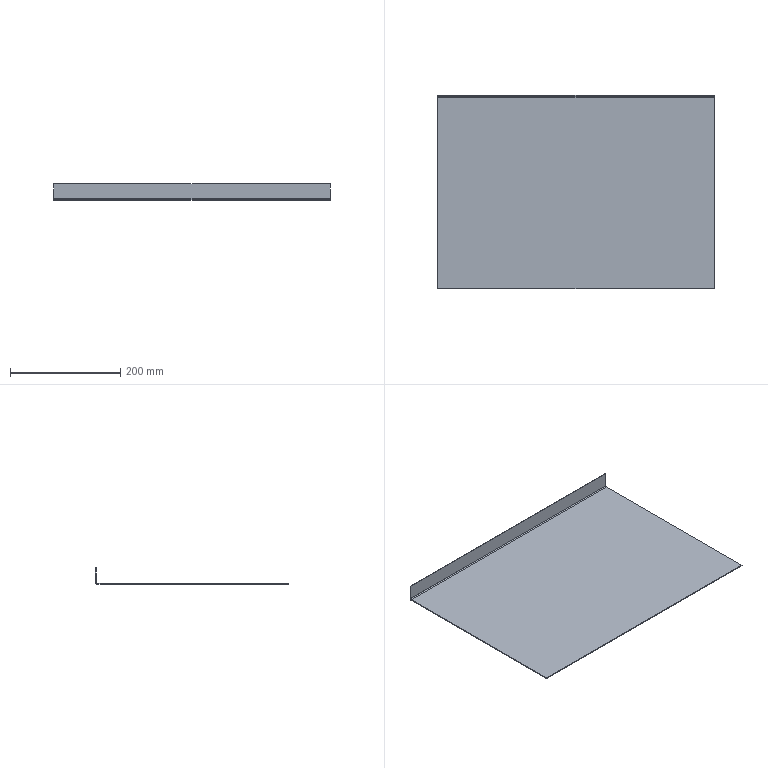Part | STEP file | SynoNew-0304-068 | 1 solid | 14 faces | box 500 x 350 x 30 mm | volume 283151 mm3 | plane 12 | cylinder 2 | commonest cylinder face diameters 3 x1 6 x1
STEP:
#1=CARTESIAN_POINT('',(250.,175.,3.));
#2=VERTEX_POINT('',#1);
#3=CARTESIAN_POINT('',(-250.,175.,3.));
#4=VERTEX_POINT('',#3);
#5=CARTESIAN_POINT('',(0.,175.,3.));
#6=DIRECTION('',(-1.,0.,0.));
#7=VECTOR('',#6,10.);
#8=LINE('',#5,#7);
#9=EDGE_CURVE('',#2,#4,#8,.T.);
#10=ORIENTED_EDGE('',*,*,#9,.F.);
#11=CARTESIAN_POINT('',(250.,172.,0.));
#12=VERTEX_POINT('',#11);
#13=CARTESIAN_POINT('',(250.,172.,3.));
#14=DIRECTION('',(1.,0.,0.));
#15=DIRECTION('',(0.,0.,-1.));
#16=AXIS2_PLACEMENT_3D('',#13,#14,#15);
#17=CIRCLE('',#16,3.);
#18=EDGE_CURVE('',#12,#2,#17,.T.);
#19=ORIENTED_EDGE('',*,*,#18,.F.);
#20=CARTESIAN_POINT('',(-250.,172.,0.));
#21=VERTEX_POINT('',#20);
#22=CARTESIAN_POINT('',(-125.,172.,0.));
#23=DIRECTION('',(1.,0.,0.));
#24=VECTOR('',#23,10.);
#25=LINE('',#22,#24);
#26=EDGE_CURVE('',#21,#12,#25,.T.);
#27=ORIENTED_EDGE('',*,*,#26,.F.);
#28=CARTESIAN_POINT('',(-250.,172.,3.));
#29=DIRECTION('',(-1.,0.,0.));
#30=DIRECTION('',(0.,1.,0.));
#31=AXIS2_PLACEMENT_3D('',#28,#29,#30);
#32=CIRCLE('',#31,3.);
#33=EDGE_CURVE('',#4,#21,#32,.T.);
#34=ORIENTED_EDGE('',*,*,#33,.F.);
#35=EDGE_LOOP('',(#10,#19,#27,#34));
#36=FACE_OUTER_BOUND('',#35,.T.);
#37=CARTESIAN_POINT('',(0.,172.,3.));
#38=DIRECTION('',(1.,0.,0.));
#39=DIRECTION('',(0.,0.,-1.));
#40=AXIS2_PLACEMENT_3D('',#37,#38,#39);
#41=CYLINDRICAL_SURFACE('',#40,3.);
#42=ADVANCED_FACE('',(#36),#41,.T.);
#43=CARTESIAN_POINT('',(-250.,173.5,3.));
#44=VERTEX_POINT('',#43);
#45=CARTESIAN_POINT('',(-250.,173.83,3.));
#46=DIRECTION('',(0.,-1.,0.));
#47=VECTOR('',#46,10.);
#48=LINE('',#45,#47);
#49=EDGE_CURVE('',#4,#44,#48,.T.);
#50=ORIENTED_EDGE('',*,*,#49,.T.);
#51=CARTESIAN_POINT('',(-250.,173.5,30.));
#52=VERTEX_POINT('',#51);
#53=CARTESIAN_POINT('',(-250.,173.5,-0.3929));
#54=DIRECTION('',(0.,0.,1.));
#55=VECTOR('',#54,10.);
#56=LINE('',#53,#55);
#57=EDGE_CURVE('',#44,#52,#56,.T.);
#58=ORIENTED_EDGE('',*,*,#57,.T.);
#59=CARTESIAN_POINT('',(-250.,175.,30.));
#60=VERTEX_POINT('',#59);
#61=CARTESIAN_POINT('',(-250.,173.5,30.));
#62=DIRECTION('',(0.,1.,0.));
#63=VECTOR('',#62,10.);
#64=LINE('',#61,#63);
#65=EDGE_CURVE('',#52,#60,#64,.T.);
#66=ORIENTED_EDGE('',*,*,#65,.T.);
#67=CARTESIAN_POINT('',(-250.,175.,-0.3929));
#68=DIRECTION('',(0.,0.,-1.));
#69=VECTOR('',#68,10.);
#70=LINE('',#67,#69);
#71=EDGE_CURVE('',#60,#4,#70,.T.);
#72=ORIENTED_EDGE('',*,*,#71,.T.);
#73=EDGE_LOOP('',(#50,#58,#66,#72));
#74=FACE_OUTER_BOUND('',#73,.T.);
#75=CARTESIAN_POINT('',(-250.,173.5,3.));
#76=DIRECTION('',(-1.,0.,0.));
#77=DIRECTION('',(0.,-1.,0.));
#78=AXIS2_PLACEMENT_3D('',#75,#76,#77);
#79=PLANE('',#78);
#80=ADVANCED_FACE('',(#74),#79,.T.);
#81=CARTESIAN_POINT('',(250.,173.5,3.));
#82=VERTEX_POINT('',#81);
#83=CARTESIAN_POINT('',(0.,173.5,3.));
#84=DIRECTION('',(1.,0.,0.));
#85=VECTOR('',#84,10.);
#86=LINE('',#83,#85);
#87=EDGE_CURVE('',#44,#82,#86,.T.);
#88=ORIENTED_EDGE('',*,*,#87,.T.);
#89=CARTESIAN_POINT('',(250.,173.5,30.));
#90=VERTEX_POINT('',#89);
#91=CARTESIAN_POINT('',(250.,173.5,-0.3929));
#92=DIRECTION('',(0.,0.,1.));
#93=VECTOR('',#92,10.);
#94=LINE('',#91,#93);
#95=EDGE_CURVE('',#82,#90,#94,.T.);
#96=ORIENTED_EDGE('',*,*,#95,.T.);
#97=CARTESIAN_POINT('',(250.,173.5,30.));
#98=DIRECTION('',(-1.,0.,0.));
#99=VECTOR('',#98,10.);
#100=LINE('',#97,#99);
#101=EDGE_CURVE('',#90,#52,#100,.T.);
#102=ORIENTED_EDGE('',*,*,#101,.T.);
#103=ORIENTED_EDGE('',*,*,#57,.F.);
#104=EDGE_LOOP('',(#88,#96,#102,#103));
#105=FACE_OUTER_BOUND('',#104,.T.);
#106=CARTESIAN_POINT('',(0.,173.5,14.804));
#107=DIRECTION('',(0.,-1.,0.));
#108=DIRECTION('',(1.,0.,0.));
#109=AXIS2_PLACEMENT_3D('',#106,#107,#108);
#110=PLANE('',#109);
#111=ADVANCED_FACE('',(#105),#110,.T.);
#112=CARTESIAN_POINT('',(250.,173.83,3.));
#113=DIRECTION('',(0.,1.,0.));
#114=VECTOR('',#113,10.);
#115=LINE('',#112,#114);
#116=EDGE_CURVE('',#82,#2,#115,.T.);
#117=ORIENTED_EDGE('',*,*,#116,.F.);
#118=CARTESIAN_POINT('',(250.,172.,1.5));
#119=VERTEX_POINT('',#118);
#120=CARTESIAN_POINT('',(250.,172.,3.));
#121=DIRECTION('',(1.,0.,0.));
#122=DIRECTION('',(0.,0.,-1.));
#123=AXIS2_PLACEMENT_3D('',#120,#121,#122);
#124=CIRCLE('',#123,1.5);
#125=EDGE_CURVE('',#119,#82,#124,.T.);
#126=ORIENTED_EDGE('',*,*,#125,.F.);
#127=CARTESIAN_POINT('',(250.,172.,0.75));
#128=DIRECTION('',(0.,0.,1.));
#129=VECTOR('',#128,10.);
#130=LINE('',#127,#129);
#131=EDGE_CURVE('',#12,#119,#130,.T.);
#132=ORIENTED_EDGE('',*,*,#131,.F.);
#133=ORIENTED_EDGE('',*,*,#18,.T.);
#134=EDGE_LOOP('',(#117,#126,#132,#133));
#135=FACE_OUTER_BOUND('',#134,.T.);
#136=CARTESIAN_POINT('',(250.,173.5,3.));
#137=DIRECTION('',(1.,0.,0.));
#138=DIRECTION('',(0.,0.,-1.));
#139=AXIS2_PLACEMENT_3D('',#136,#137,#138);
#140=PLANE('',#139);
#141=ADVANCED_FACE('',(#135),#140,.T.);
#142=ORIENTED_EDGE('',*,*,#49,.F.);
#143=ORIENTED_EDGE('',*,*,#33,.T.);
#144=CARTESIAN_POINT('',(-250.,172.,1.5));
#145=VERTEX_POINT('',#144);
#146=CARTESIAN_POINT('',(-250.,172.,0.75));
#147=DIRECTION('',(0.,0.,-1.));
#148=VECTOR('',#147,10.);
#149=LINE('',#146,#148);
#150=EDGE_CURVE('',#145,#21,#149,.T.);
#151=ORIENTED_EDGE('',*,*,#150,.F.);
#152=CARTESIAN_POINT('',(-250.,172.,3.));
#153=DIRECTION('',(1.,0.,0.));
#154=DIRECTION('',(0.,0.,-1.));
#155=AXIS2_PLACEMENT_3D('',#152,#153,#154);
#156=CIRCLE('',#155,1.5);
#157=EDGE_CURVE('',#145,#44,#156,.T.);
#158=ORIENTED_EDGE('',*,*,#157,.T.);
#159=EDGE_LOOP('',(#142,#143,#151,#158));
#160=FACE_OUTER_BOUND('',#159,.T.);
#161=CARTESIAN_POINT('',(-250.,175.,3.));
#162=DIRECTION('',(-1.,0.,0.));
#163=DIRECTION('',(0.,0.,1.));
#164=AXIS2_PLACEMENT_3D('',#161,#162,#163);
#165=PLANE('',#164);
#166=ADVANCED_FACE('',(#160),#165,.T.);
#167=ORIENTED_EDGE('',*,*,#116,.T.);
#168=CARTESIAN_POINT('',(250.,175.,30.));
#169=VERTEX_POINT('',#168);
#170=CARTESIAN_POINT('',(250.,175.,3.));
#171=DIRECTION('',(0.,0.,1.));
#172=VECTOR('',#171,10.);
#173=LINE('',#170,#172);
#174=EDGE_CURVE('',#2,#169,#173,.T.);
#175=ORIENTED_EDGE('',*,*,#174,.T.);
#176=CARTESIAN_POINT('',(250.,173.5,30.));
#177=DIRECTION('',(0.,1.,0.));
#178=VECTOR('',#177,10.);
#179=LINE('',#176,#178);
#180=EDGE_CURVE('',#90,#169,#179,.T.);
#181=ORIENTED_EDGE('',*,*,#180,.F.);
#182=ORIENTED_EDGE('',*,*,#95,.F.);
#183=EDGE_LOOP('',(#167,#175,#181,#182));
#184=FACE_OUTER_BOUND('',#183,.T.);
#185=CARTESIAN_POINT('',(250.,173.5,3.));
#186=DIRECTION('',(1.,0.,0.));
#187=DIRECTION('',(0.,1.,0.));
#188=AXIS2_PLACEMENT_3D('',#185,#186,#187);
#189=PLANE('',#188);
#190=ADVANCED_FACE('',(#184),#189,.T.);
#191=CARTESIAN_POINT('',(250.,175.,30.));
#192=DIRECTION('',(-1.,0.,0.));
#193=VECTOR('',#192,10.);
#194=LINE('',#191,#193);
#195=EDGE_CURVE('',#169,#60,#194,.T.);
#196=ORIENTED_EDGE('',*,*,#195,.T.);
#197=ORIENTED_EDGE('',*,*,#65,.F.);
#198=ORIENTED_EDGE('',*,*,#101,.F.);
#199=ORIENTED_EDGE('',*,*,#180,.T.);
#200=EDGE_LOOP('',(#196,#197,#198,#199));
#201=FACE_OUTER_BOUND('',#200,.T.);
#202=CARTESIAN_POINT('',(250.,173.5,30.));
#203=DIRECTION('',(0.,0.,1.));
#204=DIRECTION('',(0.,-1.,0.));
#205=AXIS2_PLACEMENT_3D('',#202,#203,#204);
#206=PLANE('',#205);
#207=ADVANCED_FACE('',(#201),#206,.T.);
#208=ORIENTED_EDGE('',*,*,#9,.T.);
#209=ORIENTED_EDGE('',*,*,#71,.F.);
#210=ORIENTED_EDGE('',*,*,#195,.F.);
#211=ORIENTED_EDGE('',*,*,#174,.F.);
#212=EDGE_LOOP('',(#208,#209,#210,#211));
#213=FACE_OUTER_BOUND('',#212,.T.);
#214=CARTESIAN_POINT('',(0.,175.,14.804));
#215=DIRECTION('',(0.,-1.,0.));
#216=DIRECTION('',(1.,0.,0.));
#217=AXIS2_PLACEMENT_3D('',#214,#215,#216);
#218=PLANE('',#217);
#219=ADVANCED_FACE('',(#213),#218,.F.);
#220=ORIENTED_EDGE('',*,*,#87,.F.);
#221=ORIENTED_EDGE('',*,*,#157,.F.);
#222=CARTESIAN_POINT('',(-125.,172.,1.5));
#223=DIRECTION('',(-1.,0.,0.));
#224=VECTOR('',#223,10.);
#225=LINE('',#222,#224);
#226=EDGE_CURVE('',#119,#145,#225,.T.);
#227=ORIENTED_EDGE('',*,*,#226,.F.);
#228=ORIENTED_EDGE('',*,*,#125,.T.);
#229=EDGE_LOOP('',(#220,#221,#227,#228));
#230=FACE_OUTER_BOUND('',#229,.T.);
#231=CARTESIAN_POINT('',(0.,172.,3.));
#232=DIRECTION('',(1.,0.,0.));
#233=DIRECTION('',(0.,0.,-1.));
#234=AXIS2_PLACEMENT_3D('',#231,#232,#233);
#235=CYLINDRICAL_SURFACE('',#234,1.5);
#236=ADVANCED_FACE('',(#230),#235,.F.);
#237=ORIENTED_EDGE('',*,*,#150,.T.);
#238=CARTESIAN_POINT('',(-250.,-175.,0.));
#239=VERTEX_POINT('',#238);
#240=CARTESIAN_POINT('',(-250.,-175.,0.));
#241=DIRECTION('',(0.,1.,0.));
#242=VECTOR('',#241,10.);
#243=LINE('',#240,#242);
#244=EDGE_CURVE('',#239,#21,#243,.T.);
#245=ORIENTED_EDGE('',*,*,#244,.F.);
#246=CARTESIAN_POINT('',(-250.,-175.,1.5));
#247=VERTEX_POINT('',#246);
#248=CARTESIAN_POINT('',(-250.,-175.,0.));
#249=DIRECTION('',(0.,0.,1.));
#250=VECTOR('',#249,10.);
#251=LINE('',#248,#250);
#252=EDGE_CURVE('',#239,#247,#251,.T.);
#253=ORIENTED_EDGE('',*,*,#252,.T.);
#254=CARTESIAN_POINT('',(-250.,-175.,1.5));
#255=DIRECTION('',(0.,1.,0.));
#256=VECTOR('',#255,10.);
#257=LINE('',#254,#256);
#258=EDGE_CURVE('',#247,#145,#257,.T.);
#259=ORIENTED_EDGE('',*,*,#258,.T.);
#260=EDGE_LOOP('',(#237,#245,#253,#259));
#261=FACE_OUTER_BOUND('',#260,.T.);
#262=CARTESIAN_POINT('',(-250.,-175.,0.));
#263=DIRECTION('',(-1.,0.,0.));
#264=DIRECTION('',(0.,0.,1.));
#265=AXIS2_PLACEMENT_3D('',#262,#263,#264);
#266=PLANE('',#265);
#267=ADVANCED_FACE('',(#261),#266,.T.);
#268=ORIENTED_EDGE('',*,*,#26,.T.);
#269=CARTESIAN_POINT('',(250.,-175.,0.));
#270=VERTEX_POINT('',#269);
#271=CARTESIAN_POINT('',(250.,175.,0.));
#272=DIRECTION('',(0.,-1.,0.));
#273=VECTOR('',#272,10.);
#274=LINE('',#271,#273);
#275=EDGE_CURVE('',#12,#270,#274,.T.);
#276=ORIENTED_EDGE('',*,*,#275,.T.);
#277=CARTESIAN_POINT('',(250.,-175.,0.));
#278=DIRECTION('',(-1.,0.,0.));
#279=VECTOR('',#278,10.);
#280=LINE('',#277,#279);
#281=EDGE_CURVE('',#270,#239,#280,.T.);
#282=ORIENTED_EDGE('',*,*,#281,.T.);
#283=ORIENTED_EDGE('',*,*,#244,.T.);
#284=EDGE_LOOP('',(#268,#276,#282,#283));
#285=FACE_OUTER_BOUND('',#284,.T.);
#286=CARTESIAN_POINT('',(0.,0.,0.));
#287=DIRECTION('',(0.,0.,1.));
#288=DIRECTION('',(1.,0.,0.));
#289=AXIS2_PLACEMENT_3D('',#286,#287,#288);
#290=PLANE('',#289);
#291=ADVANCED_FACE('',(#285),#290,.F.);
#292=ORIENTED_EDGE('',*,*,#131,.T.);
#293=CARTESIAN_POINT('',(250.,-175.,1.5));
#294=VERTEX_POINT('',#293);
#295=CARTESIAN_POINT('',(250.,175.,1.5));
#296=DIRECTION('',(0.,-1.,0.));
#297=VECTOR('',#296,10.);
#298=LINE('',#295,#297);
#299=EDGE_CURVE('',#119,#294,#298,.T.);
#300=ORIENTED_EDGE('',*,*,#299,.T.);
#301=CARTESIAN_POINT('',(250.,-175.,0.));
#302=DIRECTION('',(0.,0.,1.));
#303=VECTOR('',#302,10.);
#304=LINE('',#301,#303);
#305=EDGE_CURVE('',#270,#294,#304,.T.);
#306=ORIENTED_EDGE('',*,*,#305,.F.);
#307=ORIENTED_EDGE('',*,*,#275,.F.);
#308=EDGE_LOOP('',(#292,#300,#306,#307));
#309=FACE_OUTER_BOUND('',#308,.T.);
#310=CARTESIAN_POINT('',(250.,175.,0.));
#311=DIRECTION('',(1.,0.,0.));
#312=DIRECTION('',(0.,0.,-1.));
#313=AXIS2_PLACEMENT_3D('',#310,#311,#312);
#314=PLANE('',#313);
#315=ADVANCED_FACE('',(#309),#314,.T.);
#316=CARTESIAN_POINT('',(250.,-175.,1.5));
#317=DIRECTION('',(-1.,0.,0.));
#318=VECTOR('',#317,10.);
#319=LINE('',#316,#318);
#320=EDGE_CURVE('',#294,#247,#319,.T.);
#321=ORIENTED_EDGE('',*,*,#320,.T.);
#322=ORIENTED_EDGE('',*,*,#252,.F.);
#323=ORIENTED_EDGE('',*,*,#281,.F.);
#324=ORIENTED_EDGE('',*,*,#305,.T.);
#325=EDGE_LOOP('',(#321,#322,#323,#324));
#326=FACE_OUTER_BOUND('',#325,.T.);
#327=CARTESIAN_POINT('',(250.,-175.,0.));
#328=DIRECTION('',(0.,-1.,0.));
#329=DIRECTION('',(0.,0.,-1.));
#330=AXIS2_PLACEMENT_3D('',#327,#328,#329);
#331=PLANE('',#330);
#332=ADVANCED_FACE('',(#326),#331,.T.);
#333=ORIENTED_EDGE('',*,*,#226,.T.);
#334=ORIENTED_EDGE('',*,*,#258,.F.);
#335=ORIENTED_EDGE('',*,*,#320,.F.);
#336=ORIENTED_EDGE('',*,*,#299,.F.);
#337=EDGE_LOOP('',(#333,#334,#335,#336));
#338=FACE_OUTER_BOUND('',#337,.T.);
#339=CARTESIAN_POINT('',(0.,0.,1.5));
#340=DIRECTION('',(0.,0.,1.));
#341=DIRECTION('',(1.,0.,0.));
#342=AXIS2_PLACEMENT_3D('',#339,#340,#341);
#343=PLANE('',#342);
#344=ADVANCED_FACE('',(#338),#343,.T.);
#345=CLOSED_SHELL('',(#42,#80,#111,#141,#166,#190,#207,#219,#236,#267,#291,#315,#332,#344));
#346=MANIFOLD_SOLID_BREP('',#345);
#347=(LENGTH_UNIT()NAMED_UNIT(*)SI_UNIT(.MILLI.,.METRE.));
#348=UNCERTAINTY_MEASURE_WITH_UNIT(LENGTH_MEASURE(0.01),#347,'','');
#349=(NAMED_UNIT(*)PLANE_ANGLE_UNIT()SI_UNIT($,.RADIAN.));
#350=(NAMED_UNIT(*)SI_UNIT($,.STERADIAN.)SOLID_ANGLE_UNIT());
#351=(GEOMETRIC_REPRESENTATION_CONTEXT(3)GLOBAL_UNCERTAINTY_ASSIGNED_CONTEXT((#348))GLOBAL_UNIT_ASSIGNED_CONTEXT((#347,#349,#350))REPRESENTATION_CONTEXT('',''));
#352=ADVANCED_BREP_SHAPE_REPRESENTATION('',(#346),#351);